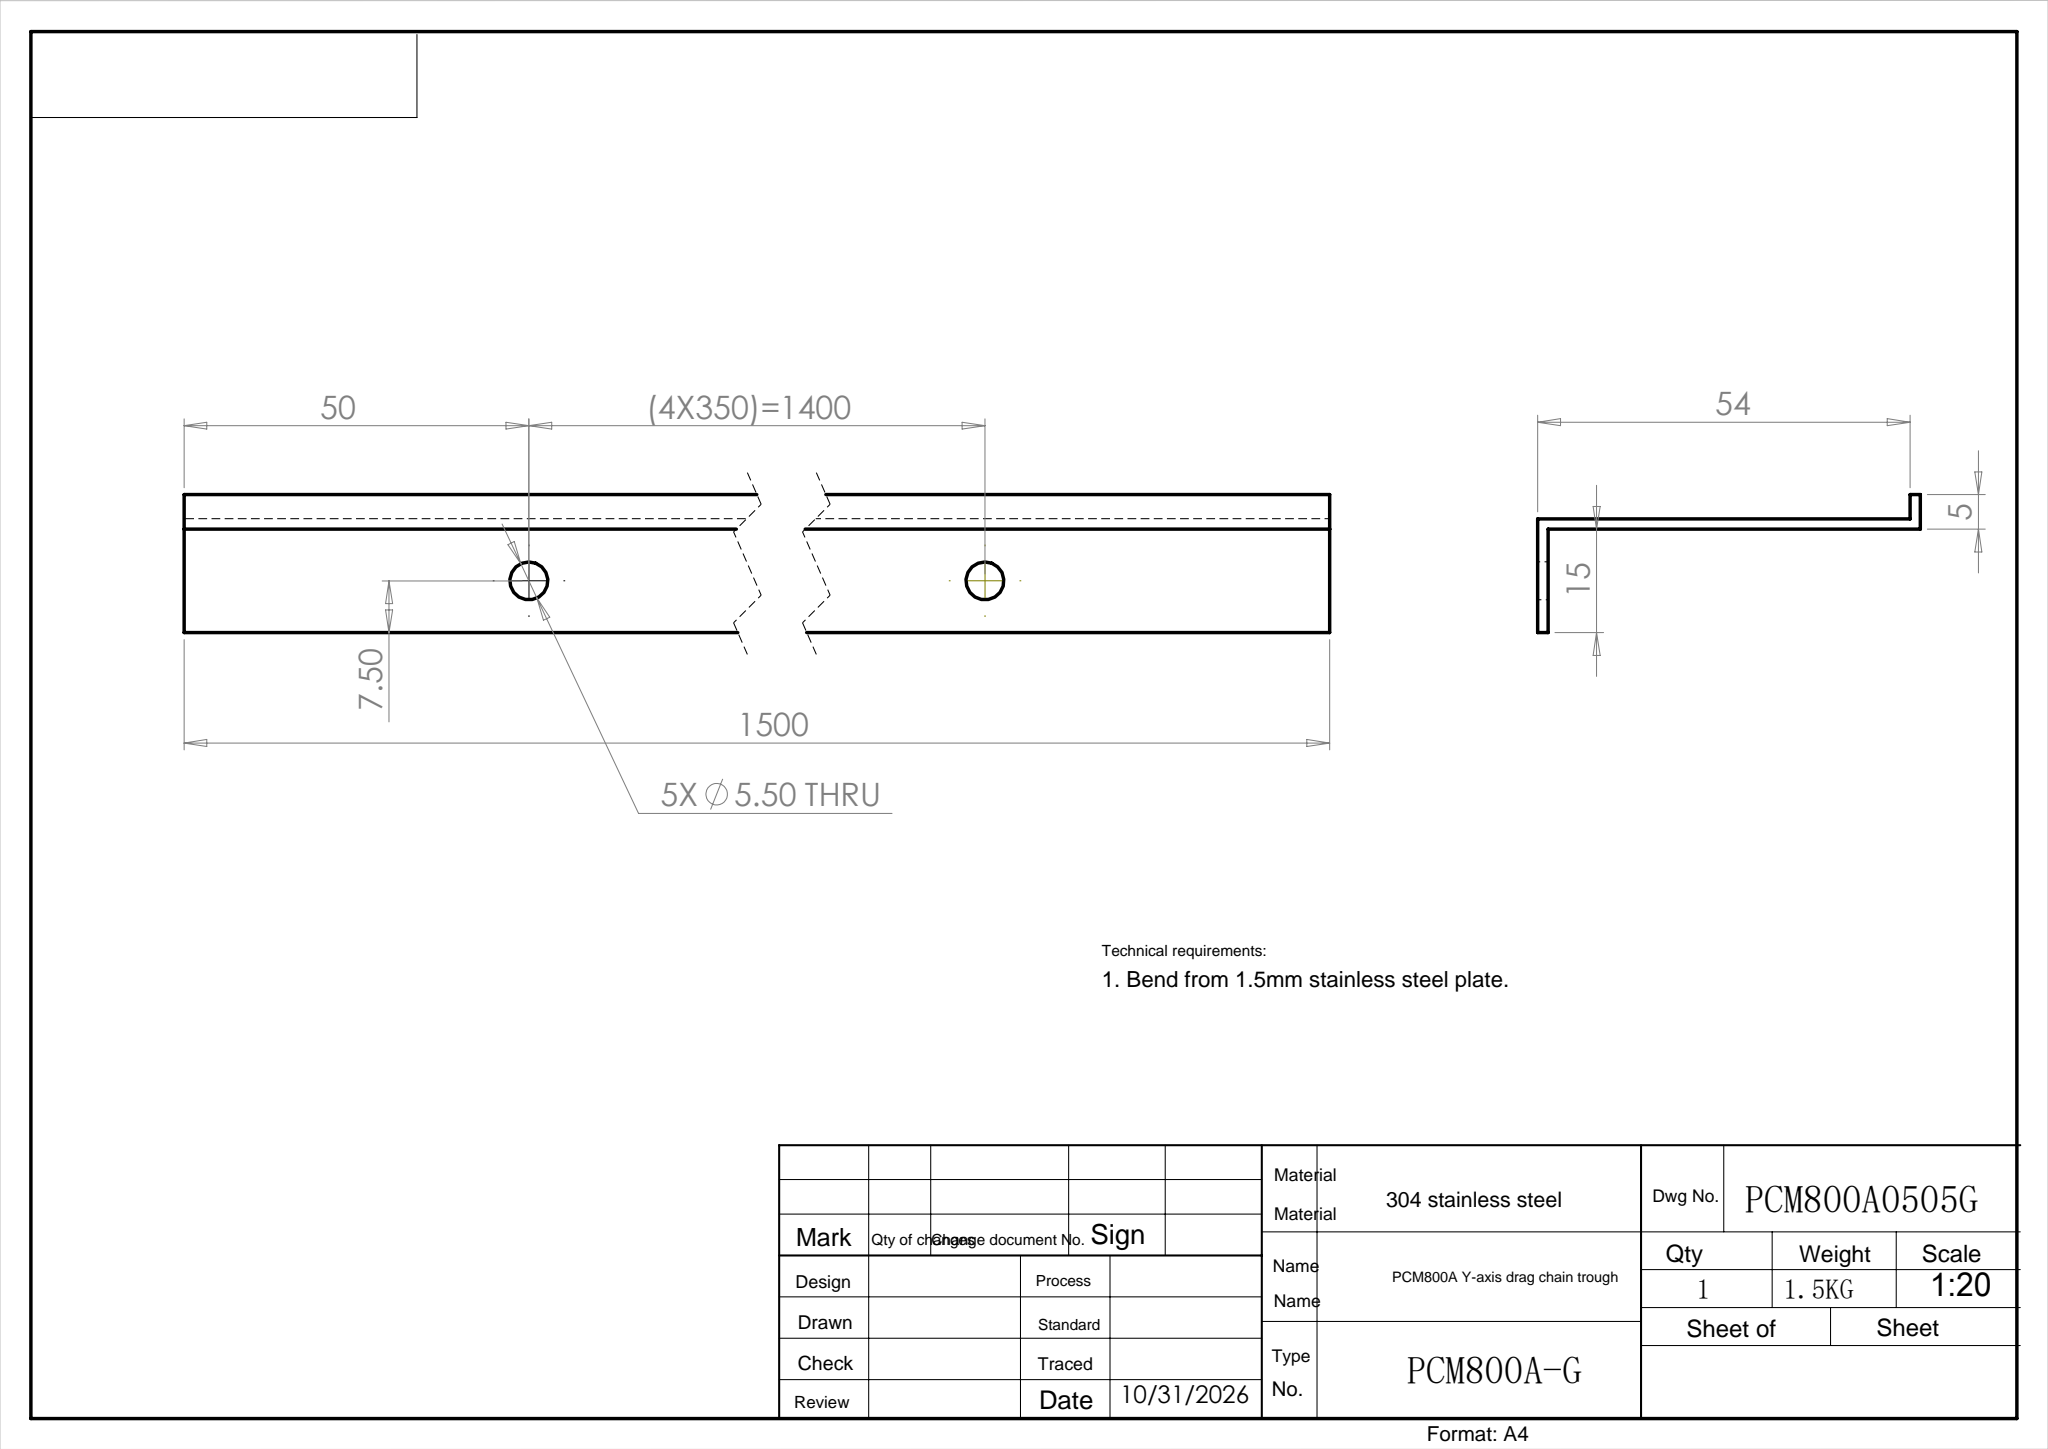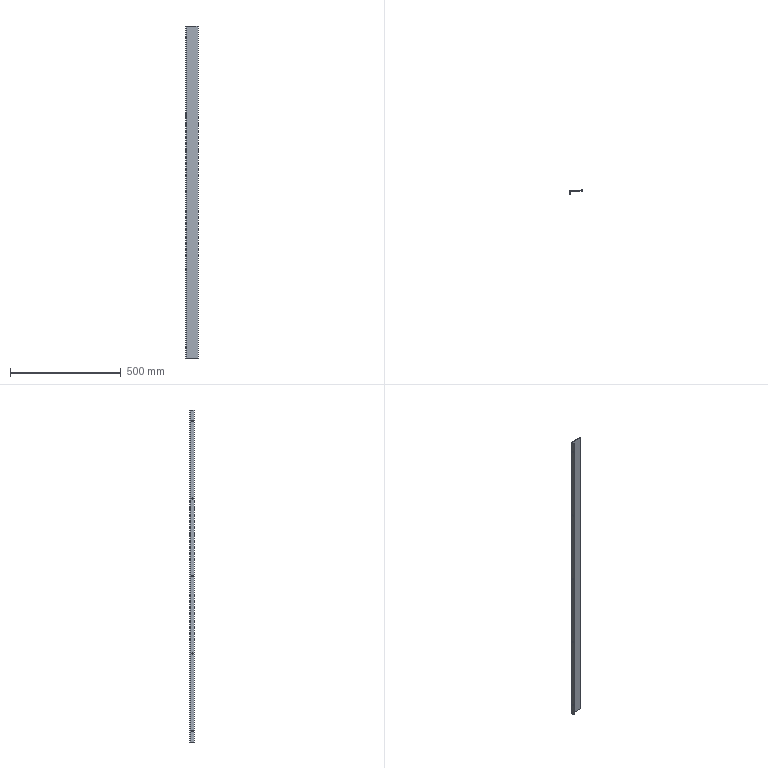Part | SolidWorks | features ExtruThin 1, ICE 1 | 1 solid | 20 faces | box 55.5 x 20 x 1500 mm | volume 166322 mm3 | cylinder 10 | plane 10 | commonest cylinder face diameters 5.5 x10
STEP:
#1=CARTESIAN_POINT('',(-1.5,-4.75,50.));
#2=VERTEX_POINT('',#1);
#3=CARTESIAN_POINT('',(-1.5,-10.25,50.));
#4=VERTEX_POINT('',#3);
#5=CARTESIAN_POINT('',(-1.5,-7.5,50.));
#6=DIRECTION('',(-1.,0.,0.));
#7=DIRECTION('',(0.,-1.,0.));
#8=AXIS2_PLACEMENT_3D('',#5,#6,#7);
#9=CIRCLE('',#8,2.75);
#10=EDGE_CURVE('',#2,#4,#9,.T.);
#11=ORIENTED_EDGE('',*,*,#10,.T.);
#12=CARTESIAN_POINT('',(0.,-10.25,50.));
#13=VERTEX_POINT('',#12);
#14=CARTESIAN_POINT('',(-10.,-10.25,50.));
#15=DIRECTION('',(1.,0.,0.));
#16=VECTOR('',#15,1000.);
#17=LINE('',#14,#16);
#18=EDGE_CURVE('',#4,#13,#17,.T.);
#19=ORIENTED_EDGE('',*,*,#18,.T.);
#20=CARTESIAN_POINT('',(0.,-4.75,50.));
#21=VERTEX_POINT('',#20);
#22=CARTESIAN_POINT('',(0.,-7.5,50.));
#23=DIRECTION('',(1.,0.,0.));
#24=DIRECTION('',(0.,1.,0.));
#25=AXIS2_PLACEMENT_3D('',#22,#23,#24);
#26=CIRCLE('',#25,2.75);
#27=EDGE_CURVE('',#13,#21,#26,.T.);
#28=ORIENTED_EDGE('',*,*,#27,.T.);
#29=CARTESIAN_POINT('',(-10.,-4.75,50.));
#30=DIRECTION('',(1.,0.,0.));
#31=VECTOR('',#30,1000.);
#32=LINE('',#29,#31);
#33=EDGE_CURVE('',#2,#21,#32,.T.);
#34=ORIENTED_EDGE('',*,*,#33,.F.);
#35=EDGE_LOOP('',(#11,#19,#28,#34));
#36=FACE_OUTER_BOUND('',#35,.T.);
#37=CARTESIAN_POINT('',(-10.,-7.5,50.));
#38=DIRECTION('',(1.,0.,0.));
#39=DIRECTION('',(0.,1.,0.));
#40=AXIS2_PLACEMENT_3D('',#37,#38,#39);
#41=CYLINDRICAL_SURFACE('',#40,2.75);
#42=ADVANCED_FACE('',(#36),#41,.F.);
#43=CARTESIAN_POINT('',(-1.5,-4.75,400.));
#44=VERTEX_POINT('',#43);
#45=CARTESIAN_POINT('',(-1.5,-10.25,400.));
#46=VERTEX_POINT('',#45);
#47=CARTESIAN_POINT('',(-1.5,-7.5,400.));
#48=DIRECTION('',(-1.,0.,0.));
#49=DIRECTION('',(0.,-1.,0.));
#50=AXIS2_PLACEMENT_3D('',#47,#48,#49);
#51=CIRCLE('',#50,2.75);
#52=EDGE_CURVE('',#44,#46,#51,.T.);
#53=ORIENTED_EDGE('',*,*,#52,.T.);
#54=CARTESIAN_POINT('',(0.,-10.25,400.));
#55=VERTEX_POINT('',#54);
#56=CARTESIAN_POINT('',(-10.,-10.25,400.));
#57=DIRECTION('',(1.,0.,0.));
#58=VECTOR('',#57,1000.);
#59=LINE('',#56,#58);
#60=EDGE_CURVE('',#46,#55,#59,.T.);
#61=ORIENTED_EDGE('',*,*,#60,.T.);
#62=CARTESIAN_POINT('',(0.,-4.75,400.));
#63=VERTEX_POINT('',#62);
#64=CARTESIAN_POINT('',(0.,-7.5,400.));
#65=DIRECTION('',(1.,0.,0.));
#66=DIRECTION('',(0.,1.,0.));
#67=AXIS2_PLACEMENT_3D('',#64,#65,#66);
#68=CIRCLE('',#67,2.75);
#69=EDGE_CURVE('',#55,#63,#68,.T.);
#70=ORIENTED_EDGE('',*,*,#69,.T.);
#71=CARTESIAN_POINT('',(-10.,-4.75,400.));
#72=DIRECTION('',(1.,0.,0.));
#73=VECTOR('',#72,1000.);
#74=LINE('',#71,#73);
#75=EDGE_CURVE('',#44,#63,#74,.T.);
#76=ORIENTED_EDGE('',*,*,#75,.F.);
#77=EDGE_LOOP('',(#53,#61,#70,#76));
#78=FACE_OUTER_BOUND('',#77,.T.);
#79=CARTESIAN_POINT('',(-10.,-7.5,400.));
#80=DIRECTION('',(1.,0.,0.));
#81=DIRECTION('',(0.,1.,0.));
#82=AXIS2_PLACEMENT_3D('',#79,#80,#81);
#83=CYLINDRICAL_SURFACE('',#82,2.75);
#84=ADVANCED_FACE('',(#78),#83,.F.);
#85=CARTESIAN_POINT('',(-1.5,-4.75,750.));
#86=VERTEX_POINT('',#85);
#87=CARTESIAN_POINT('',(-1.5,-10.25,750.));
#88=VERTEX_POINT('',#87);
#89=CARTESIAN_POINT('',(-1.5,-7.5,750.));
#90=DIRECTION('',(-1.,0.,0.));
#91=DIRECTION('',(0.,-1.,0.));
#92=AXIS2_PLACEMENT_3D('',#89,#90,#91);
#93=CIRCLE('',#92,2.75);
#94=EDGE_CURVE('',#86,#88,#93,.T.);
#95=ORIENTED_EDGE('',*,*,#94,.T.);
#96=CARTESIAN_POINT('',(0.,-10.25,750.));
#97=VERTEX_POINT('',#96);
#98=CARTESIAN_POINT('',(-10.,-10.25,750.));
#99=DIRECTION('',(1.,0.,0.));
#100=VECTOR('',#99,1000.);
#101=LINE('',#98,#100);
#102=EDGE_CURVE('',#88,#97,#101,.T.);
#103=ORIENTED_EDGE('',*,*,#102,.T.);
#104=CARTESIAN_POINT('',(0.,-4.75,750.));
#105=VERTEX_POINT('',#104);
#106=CARTESIAN_POINT('',(0.,-7.5,750.));
#107=DIRECTION('',(1.,0.,0.));
#108=DIRECTION('',(0.,1.,0.));
#109=AXIS2_PLACEMENT_3D('',#106,#107,#108);
#110=CIRCLE('',#109,2.75);
#111=EDGE_CURVE('',#97,#105,#110,.T.);
#112=ORIENTED_EDGE('',*,*,#111,.T.);
#113=CARTESIAN_POINT('',(-10.,-4.75,750.));
#114=DIRECTION('',(1.,0.,0.));
#115=VECTOR('',#114,1000.);
#116=LINE('',#113,#115);
#117=EDGE_CURVE('',#86,#105,#116,.T.);
#118=ORIENTED_EDGE('',*,*,#117,.F.);
#119=EDGE_LOOP('',(#95,#103,#112,#118));
#120=FACE_OUTER_BOUND('',#119,.T.);
#121=CARTESIAN_POINT('',(-10.,-7.5,750.));
#122=DIRECTION('',(1.,0.,0.));
#123=DIRECTION('',(0.,1.,0.));
#124=AXIS2_PLACEMENT_3D('',#121,#122,#123);
#125=CYLINDRICAL_SURFACE('',#124,2.75);
#126=ADVANCED_FACE('',(#120),#125,.F.);
#127=CARTESIAN_POINT('',(-1.5,-4.75,1100.));
#128=VERTEX_POINT('',#127);
#129=CARTESIAN_POINT('',(-1.5,-10.25,1100.));
#130=VERTEX_POINT('',#129);
#131=CARTESIAN_POINT('',(-1.5,-7.5,1100.));
#132=DIRECTION('',(-1.,0.,0.));
#133=DIRECTION('',(0.,-1.,0.));
#134=AXIS2_PLACEMENT_3D('',#131,#132,#133);
#135=CIRCLE('',#134,2.75);
#136=EDGE_CURVE('',#128,#130,#135,.T.);
#137=ORIENTED_EDGE('',*,*,#136,.T.);
#138=CARTESIAN_POINT('',(0.,-10.25,1100.));
#139=VERTEX_POINT('',#138);
#140=CARTESIAN_POINT('',(-10.,-10.25,1100.));
#141=DIRECTION('',(1.,0.,0.));
#142=VECTOR('',#141,1000.);
#143=LINE('',#140,#142);
#144=EDGE_CURVE('',#130,#139,#143,.T.);
#145=ORIENTED_EDGE('',*,*,#144,.T.);
#146=CARTESIAN_POINT('',(0.,-4.75,1100.));
#147=VERTEX_POINT('',#146);
#148=CARTESIAN_POINT('',(0.,-7.5,1100.));
#149=DIRECTION('',(1.,0.,0.));
#150=DIRECTION('',(0.,1.,0.));
#151=AXIS2_PLACEMENT_3D('',#148,#149,#150);
#152=CIRCLE('',#151,2.75);
#153=EDGE_CURVE('',#139,#147,#152,.T.);
#154=ORIENTED_EDGE('',*,*,#153,.T.);
#155=CARTESIAN_POINT('',(-10.,-4.75,1100.));
#156=DIRECTION('',(1.,0.,0.));
#157=VECTOR('',#156,1000.);
#158=LINE('',#155,#157);
#159=EDGE_CURVE('',#128,#147,#158,.T.);
#160=ORIENTED_EDGE('',*,*,#159,.F.);
#161=EDGE_LOOP('',(#137,#145,#154,#160));
#162=FACE_OUTER_BOUND('',#161,.T.);
#163=CARTESIAN_POINT('',(-10.,-7.5,1100.));
#164=DIRECTION('',(1.,0.,0.));
#165=DIRECTION('',(0.,1.,0.));
#166=AXIS2_PLACEMENT_3D('',#163,#164,#165);
#167=CYLINDRICAL_SURFACE('',#166,2.75);
#168=ADVANCED_FACE('',(#162),#167,.F.);
#169=CARTESIAN_POINT('',(-1.5,-4.75,1450.));
#170=VERTEX_POINT('',#169);
#171=CARTESIAN_POINT('',(-1.5,-10.25,1450.));
#172=VERTEX_POINT('',#171);
#173=CARTESIAN_POINT('',(-1.5,-7.5,1450.));
#174=DIRECTION('',(-1.,0.,0.));
#175=DIRECTION('',(0.,-1.,0.));
#176=AXIS2_PLACEMENT_3D('',#173,#174,#175);
#177=CIRCLE('',#176,2.75);
#178=EDGE_CURVE('',#170,#172,#177,.T.);
#179=ORIENTED_EDGE('',*,*,#178,.T.);
#180=CARTESIAN_POINT('',(0.,-10.25,1450.));
#181=VERTEX_POINT('',#180);
#182=CARTESIAN_POINT('',(-10.,-10.25,1450.));
#183=DIRECTION('',(1.,0.,0.));
#184=VECTOR('',#183,1000.);
#185=LINE('',#182,#184);
#186=EDGE_CURVE('',#172,#181,#185,.T.);
#187=ORIENTED_EDGE('',*,*,#186,.T.);
#188=CARTESIAN_POINT('',(0.,-4.75,1450.));
#189=VERTEX_POINT('',#188);
#190=CARTESIAN_POINT('',(0.,-7.5,1450.));
#191=DIRECTION('',(1.,0.,0.));
#192=DIRECTION('',(0.,1.,0.));
#193=AXIS2_PLACEMENT_3D('',#190,#191,#192);
#194=CIRCLE('',#193,2.75);
#195=EDGE_CURVE('',#181,#189,#194,.T.);
#196=ORIENTED_EDGE('',*,*,#195,.T.);
#197=CARTESIAN_POINT('',(-10.,-4.75,1450.));
#198=DIRECTION('',(1.,0.,0.));
#199=VECTOR('',#198,1000.);
#200=LINE('',#197,#199);
#201=EDGE_CURVE('',#170,#189,#200,.T.);
#202=ORIENTED_EDGE('',*,*,#201,.F.);
#203=EDGE_LOOP('',(#179,#187,#196,#202));
#204=FACE_OUTER_BOUND('',#203,.T.);
#205=CARTESIAN_POINT('',(-10.,-7.5,1450.));
#206=DIRECTION('',(1.,0.,0.));
#207=DIRECTION('',(0.,1.,0.));
#208=AXIS2_PLACEMENT_3D('',#205,#206,#207);
#209=CYLINDRICAL_SURFACE('',#208,2.75);
#210=ADVANCED_FACE('',(#204),#209,.F.);
#211=CARTESIAN_POINT('',(54.,0.,0.));
#212=VERTEX_POINT('',#211);
#213=CARTESIAN_POINT('',(54.,5.,0.));
#214=VERTEX_POINT('',#213);
#215=CARTESIAN_POINT('',(54.,0.,0.));
#216=DIRECTION('',(0.,1.,0.));
#217=VECTOR('',#216,1000.);
#218=LINE('',#215,#217);
#219=EDGE_CURVE('',#212,#214,#218,.T.);
#220=ORIENTED_EDGE('',*,*,#219,.T.);
#221=CARTESIAN_POINT('',(54.,5.,1500.));
#222=VERTEX_POINT('',#221);
#223=CARTESIAN_POINT('',(54.,5.,1500.));
#224=DIRECTION('',(0.,0.,-1.));
#225=VECTOR('',#224,1000.);
#226=LINE('',#223,#225);
#227=EDGE_CURVE('',#222,#214,#226,.T.);
#228=ORIENTED_EDGE('',*,*,#227,.F.);
#229=CARTESIAN_POINT('',(54.,0.,1500.));
#230=VERTEX_POINT('',#229);
#231=CARTESIAN_POINT('',(54.,0.,1500.));
#232=DIRECTION('',(0.,1.,0.));
#233=VECTOR('',#232,1000.);
#234=LINE('',#231,#233);
#235=EDGE_CURVE('',#230,#222,#234,.T.);
#236=ORIENTED_EDGE('',*,*,#235,.F.);
#237=CARTESIAN_POINT('',(54.,0.,1500.));
#238=DIRECTION('',(0.,0.,-1.));
#239=VECTOR('',#238,1000.);
#240=LINE('',#237,#239);
#241=EDGE_CURVE('',#230,#212,#240,.T.);
#242=ORIENTED_EDGE('',*,*,#241,.T.);
#243=EDGE_LOOP('',(#220,#228,#236,#242));
#244=FACE_OUTER_BOUND('',#243,.T.);
#245=CARTESIAN_POINT('',(54.,0.,1500.));
#246=DIRECTION('',(-1.,0.,0.));
#247=DIRECTION('',(0.,0.,1.));
#248=AXIS2_PLACEMENT_3D('',#245,#246,#247);
#249=PLANE('',#248);
#250=ADVANCED_FACE('',(#244),#249,.F.);
#251=CARTESIAN_POINT('',(52.5,5.,0.));
#252=VERTEX_POINT('',#251);
#253=CARTESIAN_POINT('',(52.5,5.,0.));
#254=DIRECTION('',(1.,0.,0.));
#255=VECTOR('',#254,1000.);
#256=LINE('',#253,#255);
#257=EDGE_CURVE('',#252,#214,#256,.T.);
#258=ORIENTED_EDGE('',*,*,#257,.F.);
#259=CARTESIAN_POINT('',(52.5,5.,1500.));
#260=VERTEX_POINT('',#259);
#261=CARTESIAN_POINT('',(52.5,5.,1500.));
#262=DIRECTION('',(0.,0.,-1.));
#263=VECTOR('',#262,1000.);
#264=LINE('',#261,#263);
#265=EDGE_CURVE('',#260,#252,#264,.T.);
#266=ORIENTED_EDGE('',*,*,#265,.F.);
#267=CARTESIAN_POINT('',(52.5,5.,1500.));
#268=DIRECTION('',(1.,0.,0.));
#269=VECTOR('',#268,1000.);
#270=LINE('',#267,#269);
#271=EDGE_CURVE('',#260,#222,#270,.T.);
#272=ORIENTED_EDGE('',*,*,#271,.T.);
#273=ORIENTED_EDGE('',*,*,#227,.T.);
#274=EDGE_LOOP('',(#258,#266,#272,#273));
#275=FACE_OUTER_BOUND('',#274,.T.);
#276=CARTESIAN_POINT('',(52.5,5.,1500.));
#277=DIRECTION('',(0.,1.,0.));
#278=DIRECTION('',(0.,0.,1.));
#279=AXIS2_PLACEMENT_3D('',#276,#277,#278);
#280=PLANE('',#279);
#281=ADVANCED_FACE('',(#275),#280,.T.);
#282=CARTESIAN_POINT('',(52.5,1.5,0.));
#283=VERTEX_POINT('',#282);
#284=CARTESIAN_POINT('',(52.5,0.,0.));
#285=DIRECTION('',(0.,1.,0.));
#286=VECTOR('',#285,1000.);
#287=LINE('',#284,#286);
#288=EDGE_CURVE('',#283,#252,#287,.T.);
#289=ORIENTED_EDGE('',*,*,#288,.F.);
#290=CARTESIAN_POINT('',(52.5,1.5,1500.));
#291=VERTEX_POINT('',#290);
#292=CARTESIAN_POINT('',(52.5,1.5,1500.));
#293=DIRECTION('',(0.,0.,-1.));
#294=VECTOR('',#293,1000.);
#295=LINE('',#292,#294);
#296=EDGE_CURVE('',#291,#283,#295,.T.);
#297=ORIENTED_EDGE('',*,*,#296,.F.);
#298=CARTESIAN_POINT('',(52.5,0.,1500.));
#299=DIRECTION('',(0.,1.,0.));
#300=VECTOR('',#299,1000.);
#301=LINE('',#298,#300);
#302=EDGE_CURVE('',#291,#260,#301,.T.);
#303=ORIENTED_EDGE('',*,*,#302,.T.);
#304=ORIENTED_EDGE('',*,*,#265,.T.);
#305=EDGE_LOOP('',(#289,#297,#303,#304));
#306=FACE_OUTER_BOUND('',#305,.T.);
#307=CARTESIAN_POINT('',(52.5,0.,1500.));
#308=DIRECTION('',(-1.,0.,0.));
#309=DIRECTION('',(0.,0.,1.));
#310=AXIS2_PLACEMENT_3D('',#307,#308,#309);
#311=PLANE('',#310);
#312=ADVANCED_FACE('',(#306),#311,.T.);
#313=CARTESIAN_POINT('',(-1.5,1.5,0.));
#314=VERTEX_POINT('',#313);
#315=CARTESIAN_POINT('',(0.,1.5,0.));
#316=DIRECTION('',(1.,0.,0.));
#317=VECTOR('',#316,1000.);
#318=LINE('',#315,#317);
#319=EDGE_CURVE('',#314,#283,#318,.T.);
#320=ORIENTED_EDGE('',*,*,#319,.F.);
#321=CARTESIAN_POINT('',(-1.5,1.5,1500.));
#322=VERTEX_POINT('',#321);
#323=CARTESIAN_POINT('',(-1.5,1.5,1500.));
#324=DIRECTION('',(0.,0.,-1.));
#325=VECTOR('',#324,1000.);
#326=LINE('',#323,#325);
#327=EDGE_CURVE('',#322,#314,#326,.T.);
#328=ORIENTED_EDGE('',*,*,#327,.F.);
#329=CARTESIAN_POINT('',(0.,1.5,1500.));
#330=DIRECTION('',(1.,0.,0.));
#331=VECTOR('',#330,1000.);
#332=LINE('',#329,#331);
#333=EDGE_CURVE('',#322,#291,#332,.T.);
#334=ORIENTED_EDGE('',*,*,#333,.T.);
#335=ORIENTED_EDGE('',*,*,#296,.T.);
#336=EDGE_LOOP('',(#320,#328,#334,#335));
#337=FACE_OUTER_BOUND('',#336,.T.);
#338=CARTESIAN_POINT('',(0.,1.5,1500.));
#339=DIRECTION('',(0.,1.,0.));
#340=DIRECTION('',(0.,0.,1.));
#341=AXIS2_PLACEMENT_3D('',#338,#339,#340);
#342=PLANE('',#341);
#343=ADVANCED_FACE('',(#337),#342,.T.);
#344=ORIENTED_EDGE('',*,*,#10,.F.);
#345=CARTESIAN_POINT('',(-1.5,-7.5,50.));
#346=DIRECTION('',(-1.,0.,0.));
#347=DIRECTION('',(0.,-1.,0.));
#348=AXIS2_PLACEMENT_3D('',#345,#346,#347);
#349=CIRCLE('',#348,2.75);
#350=EDGE_CURVE('',#4,#2,#349,.T.);
#351=ORIENTED_EDGE('',*,*,#350,.F.);
#352=EDGE_LOOP('',(#344,#351));
#353=FACE_BOUND('',#352,.T.);
#354=ORIENTED_EDGE('',*,*,#52,.F.);
#355=CARTESIAN_POINT('',(-1.5,-7.5,400.));
#356=DIRECTION('',(-1.,0.,0.));
#357=DIRECTION('',(0.,-1.,0.));
#358=AXIS2_PLACEMENT_3D('',#355,#356,#357);
#359=CIRCLE('',#358,2.75);
#360=EDGE_CURVE('',#46,#44,#359,.T.);
#361=ORIENTED_EDGE('',*,*,#360,.F.);
#362=EDGE_LOOP('',(#354,#361));
#363=FACE_BOUND('',#362,.T.);
#364=ORIENTED_EDGE('',*,*,#94,.F.);
#365=CARTESIAN_POINT('',(-1.5,-7.5,750.));
#366=DIRECTION('',(-1.,0.,0.));
#367=DIRECTION('',(0.,-1.,0.));
#368=AXIS2_PLACEMENT_3D('',#365,#366,#367);
#369=CIRCLE('',#368,2.75);
#370=EDGE_CURVE('',#88,#86,#369,.T.);
#371=ORIENTED_EDGE('',*,*,#370,.F.);
#372=EDGE_LOOP('',(#364,#371));
#373=FACE_BOUND('',#372,.T.);
#374=ORIENTED_EDGE('',*,*,#136,.F.);
#375=CARTESIAN_POINT('',(-1.5,-7.5,1100.));
#376=DIRECTION('',(-1.,0.,0.));
#377=DIRECTION('',(0.,-1.,0.));
#378=AXIS2_PLACEMENT_3D('',#375,#376,#377);
#379=CIRCLE('',#378,2.75);
#380=EDGE_CURVE('',#130,#128,#379,.T.);
#381=ORIENTED_EDGE('',*,*,#380,.F.);
#382=EDGE_LOOP('',(#374,#381));
#383=FACE_BOUND('',#382,.T.);
#384=ORIENTED_EDGE('',*,*,#178,.F.);
#385=CARTESIAN_POINT('',(-1.5,-7.5,1450.));
#386=DIRECTION('',(-1.,0.,0.));
#387=DIRECTION('',(0.,-1.,0.));
#388=AXIS2_PLACEMENT_3D('',#385,#386,#387);
#389=CIRCLE('',#388,2.75);
#390=EDGE_CURVE('',#172,#170,#389,.T.);
#391=ORIENTED_EDGE('',*,*,#390,.F.);
#392=EDGE_LOOP('',(#384,#391));
#393=FACE_BOUND('',#392,.T.);
#394=CARTESIAN_POINT('',(-1.5,-15.,0.));
#395=VERTEX_POINT('',#394);
#396=CARTESIAN_POINT('',(-1.5,0.,0.));
#397=DIRECTION('',(0.,1.,0.));
#398=VECTOR('',#397,1000.);
#399=LINE('',#396,#398);
#400=EDGE_CURVE('',#395,#314,#399,.T.);
#401=ORIENTED_EDGE('',*,*,#400,.F.);
#402=CARTESIAN_POINT('',(-1.5,-15.,1500.));
#403=VERTEX_POINT('',#402);
#404=CARTESIAN_POINT('',(-1.5,-15.,1500.));
#405=DIRECTION('',(0.,0.,-1.));
#406=VECTOR('',#405,1000.);
#407=LINE('',#404,#406);
#408=EDGE_CURVE('',#403,#395,#407,.T.);
#409=ORIENTED_EDGE('',*,*,#408,.F.);
#410=CARTESIAN_POINT('',(-1.5,0.,1500.));
#411=DIRECTION('',(0.,1.,0.));
#412=VECTOR('',#411,1000.);
#413=LINE('',#410,#412);
#414=EDGE_CURVE('',#403,#322,#413,.T.);
#415=ORIENTED_EDGE('',*,*,#414,.T.);
#416=ORIENTED_EDGE('',*,*,#327,.T.);
#417=EDGE_LOOP('',(#401,#409,#415,#416));
#418=FACE_OUTER_BOUND('',#417,.T.);
#419=CARTESIAN_POINT('',(-1.5,0.,1500.));
#420=DIRECTION('',(-1.,0.,0.));
#421=DIRECTION('',(0.,-1.,0.));
#422=AXIS2_PLACEMENT_3D('',#419,#420,#421);
#423=PLANE('',#422);
#424=ADVANCED_FACE('',(#353,#363,#373,#383,#393,#418),#423,.T.);
#425=CARTESIAN_POINT('',(0.,-15.,0.));
#426=VERTEX_POINT('',#425);
#427=CARTESIAN_POINT('',(0.,-15.,0.));
#428=DIRECTION('',(-1.,0.,0.));
#429=VECTOR('',#428,1000.);
#430=LINE('',#427,#429);
#431=EDGE_CURVE('',#426,#395,#430,.T.);
#432=ORIENTED_EDGE('',*,*,#431,.F.);
#433=CARTESIAN_POINT('',(0.,-15.,1500.));
#434=VERTEX_POINT('',#433);
#435=CARTESIAN_POINT('',(0.,-15.,1500.));
#436=DIRECTION('',(0.,0.,-1.));
#437=VECTOR('',#436,1000.);
#438=LINE('',#435,#437);
#439=EDGE_CURVE('',#434,#426,#438,.T.);
#440=ORIENTED_EDGE('',*,*,#439,.F.);
#441=CARTESIAN_POINT('',(0.,-15.,1500.));
#442=DIRECTION('',(-1.,0.,0.));
#443=VECTOR('',#442,1000.);
#444=LINE('',#441,#443);
#445=EDGE_CURVE('',#434,#403,#444,.T.);
#446=ORIENTED_EDGE('',*,*,#445,.T.);
#447=ORIENTED_EDGE('',*,*,#408,.T.);
#448=EDGE_LOOP('',(#432,#440,#446,#447));
#449=FACE_OUTER_BOUND('',#448,.T.);
#450=CARTESIAN_POINT('',(0.,-15.,1500.));
#451=DIRECTION('',(0.,-1.,0.));
#452=DIRECTION('',(0.,0.,-1.));
#453=AXIS2_PLACEMENT_3D('',#450,#451,#452);
#454=PLANE('',#453);
#455=ADVANCED_FACE('',(#449),#454,.T.);
#456=CARTESIAN_POINT('',(0.,-7.5,50.));
#457=DIRECTION('',(1.,0.,0.));
#458=DIRECTION('',(0.,1.,0.));
#459=AXIS2_PLACEMENT_3D('',#456,#457,#458);
#460=CIRCLE('',#459,2.75);
#461=EDGE_CURVE('',#21,#13,#460,.T.);
#462=ORIENTED_EDGE('',*,*,#461,.F.);
#463=ORIENTED_EDGE('',*,*,#27,.F.);
#464=EDGE_LOOP('',(#462,#463));
#465=FACE_BOUND('',#464,.T.);
#466=CARTESIAN_POINT('',(0.,-7.5,400.));
#467=DIRECTION('',(1.,0.,0.));
#468=DIRECTION('',(0.,1.,0.));
#469=AXIS2_PLACEMENT_3D('',#466,#467,#468);
#470=CIRCLE('',#469,2.75);
#471=EDGE_CURVE('',#63,#55,#470,.T.);
#472=ORIENTED_EDGE('',*,*,#471,.F.);
#473=ORIENTED_EDGE('',*,*,#69,.F.);
#474=EDGE_LOOP('',(#472,#473));
#475=FACE_BOUND('',#474,.T.);
#476=CARTESIAN_POINT('',(0.,-7.5,750.));
#477=DIRECTION('',(1.,0.,0.));
#478=DIRECTION('',(0.,1.,0.));
#479=AXIS2_PLACEMENT_3D('',#476,#477,#478);
#480=CIRCLE('',#479,2.75);
#481=EDGE_CURVE('',#105,#97,#480,.T.);
#482=ORIENTED_EDGE('',*,*,#481,.F.);
#483=ORIENTED_EDGE('',*,*,#111,.F.);
#484=EDGE_LOOP('',(#482,#483));
#485=FACE_BOUND('',#484,.T.);
#486=CARTESIAN_POINT('',(0.,-7.5,1100.));
#487=DIRECTION('',(1.,0.,0.));
#488=DIRECTION('',(0.,1.,0.));
#489=AXIS2_PLACEMENT_3D('',#486,#487,#488);
#490=CIRCLE('',#489,2.75);
#491=EDGE_CURVE('',#147,#139,#490,.T.);
#492=ORIENTED_EDGE('',*,*,#491,.F.);
#493=ORIENTED_EDGE('',*,*,#153,.F.);
#494=EDGE_LOOP('',(#492,#493));
#495=FACE_BOUND('',#494,.T.);
#496=CARTESIAN_POINT('',(0.,-7.5,1450.));
#497=DIRECTION('',(1.,0.,0.));
#498=DIRECTION('',(0.,1.,0.));
#499=AXIS2_PLACEMENT_3D('',#496,#497,#498);
#500=CIRCLE('',#499,2.75);
#501=EDGE_CURVE('',#189,#181,#500,.T.);
#502=ORIENTED_EDGE('',*,*,#501,.F.);
#503=ORIENTED_EDGE('',*,*,#195,.F.);
#504=EDGE_LOOP('',(#502,#503));
#505=FACE_BOUND('',#504,.T.);
#506=CARTESIAN_POINT('',(0.,0.,0.));
#507=VERTEX_POINT('',#506);
#508=CARTESIAN_POINT('',(0.,0.,0.));
#509=DIRECTION('',(0.,1.,0.));
#510=VECTOR('',#509,1000.);
#511=LINE('',#508,#510);
#512=EDGE_CURVE('',#426,#507,#511,.T.);
#513=ORIENTED_EDGE('',*,*,#512,.T.);
#514=CARTESIAN_POINT('',(0.,0.,1500.));
#515=VERTEX_POINT('',#514);
#516=CARTESIAN_POINT('',(0.,0.,1500.));
#517=DIRECTION('',(0.,0.,-1.));
#518=VECTOR('',#517,1000.);
#519=LINE('',#516,#518);
#520=EDGE_CURVE('',#515,#507,#519,.T.);
#521=ORIENTED_EDGE('',*,*,#520,.F.);
#522=CARTESIAN_POINT('',(0.,0.,1500.));
#523=DIRECTION('',(0.,1.,0.));
#524=VECTOR('',#523,1000.);
#525=LINE('',#522,#524);
#526=EDGE_CURVE('',#434,#515,#525,.T.);
#527=ORIENTED_EDGE('',*,*,#526,.F.);
#528=ORIENTED_EDGE('',*,*,#439,.T.);
#529=EDGE_LOOP('',(#513,#521,#527,#528));
#530=FACE_OUTER_BOUND('',#529,.T.);
#531=CARTESIAN_POINT('',(0.,0.,1500.));
#532=DIRECTION('',(-1.,0.,0.));
#533=DIRECTION('',(0.,-1.,0.));
#534=AXIS2_PLACEMENT_3D('',#531,#532,#533);
#535=PLANE('',#534);
#536=ADVANCED_FACE('',(#465,#475,#485,#495,#505,#530),#535,.F.);
#537=CARTESIAN_POINT('',(0.,0.,0.));
#538=DIRECTION('',(1.,0.,0.));
#539=VECTOR('',#538,1000.);
#540=LINE('',#537,#539);
#541=EDGE_CURVE('',#507,#212,#540,.T.);
#542=ORIENTED_EDGE('',*,*,#541,.T.);
#543=ORIENTED_EDGE('',*,*,#241,.F.);
#544=CARTESIAN_POINT('',(0.,0.,1500.));
#545=DIRECTION('',(1.,0.,0.));
#546=VECTOR('',#545,1000.);
#547=LINE('',#544,#546);
#548=EDGE_CURVE('',#515,#230,#547,.T.);
#549=ORIENTED_EDGE('',*,*,#548,.F.);
#550=ORIENTED_EDGE('',*,*,#520,.T.);
#551=EDGE_LOOP('',(#542,#543,#549,#550));
#552=FACE_OUTER_BOUND('',#551,.T.);
#553=CARTESIAN_POINT('',(0.,0.,1500.));
#554=DIRECTION('',(0.,1.,0.));
#555=DIRECTION('',(0.,0.,1.));
#556=AXIS2_PLACEMENT_3D('',#553,#554,#555);
#557=PLANE('',#556);
#558=ADVANCED_FACE('',(#552),#557,.F.);
#559=ORIENTED_EDGE('',*,*,#235,.T.);
#560=ORIENTED_EDGE('',*,*,#271,.F.);
#561=ORIENTED_EDGE('',*,*,#302,.F.);
#562=ORIENTED_EDGE('',*,*,#333,.F.);
#563=ORIENTED_EDGE('',*,*,#414,.F.);
#564=ORIENTED_EDGE('',*,*,#445,.F.);
#565=ORIENTED_EDGE('',*,*,#526,.T.);
#566=ORIENTED_EDGE('',*,*,#548,.T.);
#567=EDGE_LOOP('',(#559,#560,#561,#562,#563,#564,#565,#566));
#568=FACE_OUTER_BOUND('',#567,.T.);
#569=CARTESIAN_POINT('',(54.,5.,1500.));
#570=DIRECTION('',(0.,0.,-1.));
#571=DIRECTION('',(-1.,0.,0.));
#572=AXIS2_PLACEMENT_3D('',#569,#570,#571);
#573=PLANE('',#572);
#574=ADVANCED_FACE('',(#568),#573,.F.);
#575=ORIENTED_EDGE('',*,*,#219,.F.);
#576=ORIENTED_EDGE('',*,*,#541,.F.);
#577=ORIENTED_EDGE('',*,*,#512,.F.);
#578=ORIENTED_EDGE('',*,*,#431,.T.);
#579=ORIENTED_EDGE('',*,*,#400,.T.);
#580=ORIENTED_EDGE('',*,*,#319,.T.);
#581=ORIENTED_EDGE('',*,*,#288,.T.);
#582=ORIENTED_EDGE('',*,*,#257,.T.);
#583=EDGE_LOOP('',(#575,#576,#577,#578,#579,#580,#581,#582));
#584=FACE_OUTER_BOUND('',#583,.T.);
#585=CARTESIAN_POINT('',(54.,5.,0.));
#586=DIRECTION('',(0.,0.,-1.));
#587=DIRECTION('',(-1.,0.,0.));
#588=AXIS2_PLACEMENT_3D('',#585,#586,#587);
#589=PLANE('',#588);
#590=ADVANCED_FACE('',(#584),#589,.T.);
#591=ORIENTED_EDGE('',*,*,#186,.F.);
#592=ORIENTED_EDGE('',*,*,#390,.T.);
#593=ORIENTED_EDGE('',*,*,#201,.T.);
#594=ORIENTED_EDGE('',*,*,#501,.T.);
#595=EDGE_LOOP('',(#591,#592,#593,#594));
#596=FACE_OUTER_BOUND('',#595,.T.);
#597=CARTESIAN_POINT('',(-10.,-7.5,1450.));
#598=DIRECTION('',(1.,0.,0.));
#599=DIRECTION('',(0.,1.,0.));
#600=AXIS2_PLACEMENT_3D('',#597,#598,#599);
#601=CYLINDRICAL_SURFACE('',#600,2.75);
#602=ADVANCED_FACE('',(#596),#601,.F.);
#603=ORIENTED_EDGE('',*,*,#144,.F.);
#604=ORIENTED_EDGE('',*,*,#380,.T.);
#605=ORIENTED_EDGE('',*,*,#159,.T.);
#606=ORIENTED_EDGE('',*,*,#491,.T.);
#607=EDGE_LOOP('',(#603,#604,#605,#606));
#608=FACE_OUTER_BOUND('',#607,.T.);
#609=CARTESIAN_POINT('',(-10.,-7.5,1100.));
#610=DIRECTION('',(1.,0.,0.));
#611=DIRECTION('',(0.,1.,0.));
#612=AXIS2_PLACEMENT_3D('',#609,#610,#611);
#613=CYLINDRICAL_SURFACE('',#612,2.75);
#614=ADVANCED_FACE('',(#608),#613,.F.);
#615=ORIENTED_EDGE('',*,*,#102,.F.);
#616=ORIENTED_EDGE('',*,*,#370,.T.);
#617=ORIENTED_EDGE('',*,*,#117,.T.);
#618=ORIENTED_EDGE('',*,*,#481,.T.);
#619=EDGE_LOOP('',(#615,#616,#617,#618));
#620=FACE_OUTER_BOUND('',#619,.T.);
#621=CARTESIAN_POINT('',(-10.,-7.5,750.));
#622=DIRECTION('',(1.,0.,0.));
#623=DIRECTION('',(0.,1.,0.));
#624=AXIS2_PLACEMENT_3D('',#621,#622,#623);
#625=CYLINDRICAL_SURFACE('',#624,2.75);
#626=ADVANCED_FACE('',(#620),#625,.F.);
#627=ORIENTED_EDGE('',*,*,#60,.F.);
#628=ORIENTED_EDGE('',*,*,#360,.T.);
#629=ORIENTED_EDGE('',*,*,#75,.T.);
#630=ORIENTED_EDGE('',*,*,#471,.T.);
#631=EDGE_LOOP('',(#627,#628,#629,#630));
#632=FACE_OUTER_BOUND('',#631,.T.);
#633=CARTESIAN_POINT('',(-10.,-7.5,400.));
#634=DIRECTION('',(1.,0.,0.));
#635=DIRECTION('',(0.,1.,0.));
#636=AXIS2_PLACEMENT_3D('',#633,#634,#635);
#637=CYLINDRICAL_SURFACE('',#636,2.75);
#638=ADVANCED_FACE('',(#632),#637,.F.);
#639=ORIENTED_EDGE('',*,*,#18,.F.);
#640=ORIENTED_EDGE('',*,*,#350,.T.);
#641=ORIENTED_EDGE('',*,*,#33,.T.);
#642=ORIENTED_EDGE('',*,*,#461,.T.);
#643=EDGE_LOOP('',(#639,#640,#641,#642));
#644=FACE_OUTER_BOUND('',#643,.T.);
#645=CARTESIAN_POINT('',(-10.,-7.5,50.));
#646=DIRECTION('',(1.,0.,0.));
#647=DIRECTION('',(0.,1.,0.));
#648=AXIS2_PLACEMENT_3D('',#645,#646,#647);
#649=CYLINDRICAL_SURFACE('',#648,2.75);
#650=ADVANCED_FACE('',(#644),#649,.F.);
#651=CLOSED_SHELL('',(#42,#84,#126,#168,#210,#250,#281,#312,#343,#424,#455,#536,#558,#574,#590,#602,#614,#626,#638,#650));
#652=MANIFOLD_SOLID_BREP('',#651);
#653=CARTESIAN_POINT('',(0.,0.,0.));
#654=DIRECTION('',(0.,0.,1.));
#655=DIRECTION('',(1.,0.,0.));
#656=AXIS2_PLACEMENT_3D('',#653,#654,#655);
#657=(LENGTH_UNIT()NAMED_UNIT(*)SI_UNIT(.MILLI.,.METRE.));
#658=UNCERTAINTY_MEASURE_WITH_UNIT(LENGTH_MEASURE(0.00001),#657,'','');
#659=(NAMED_UNIT(*)PLANE_ANGLE_UNIT()SI_UNIT($,.RADIAN.));
#660=(NAMED_UNIT(*)SI_UNIT($,.STERADIAN.)SOLID_ANGLE_UNIT());
#661=(GEOMETRIC_REPRESENTATION_CONTEXT(3)GLOBAL_UNCERTAINTY_ASSIGNED_CONTEXT((#658))GLOBAL_UNIT_ASSIGNED_CONTEXT((#657,#659,#660))REPRESENTATION_CONTEXT('',''));
#662=ADVANCED_BREP_SHAPE_REPRESENTATION('',(#652,#656),#661);